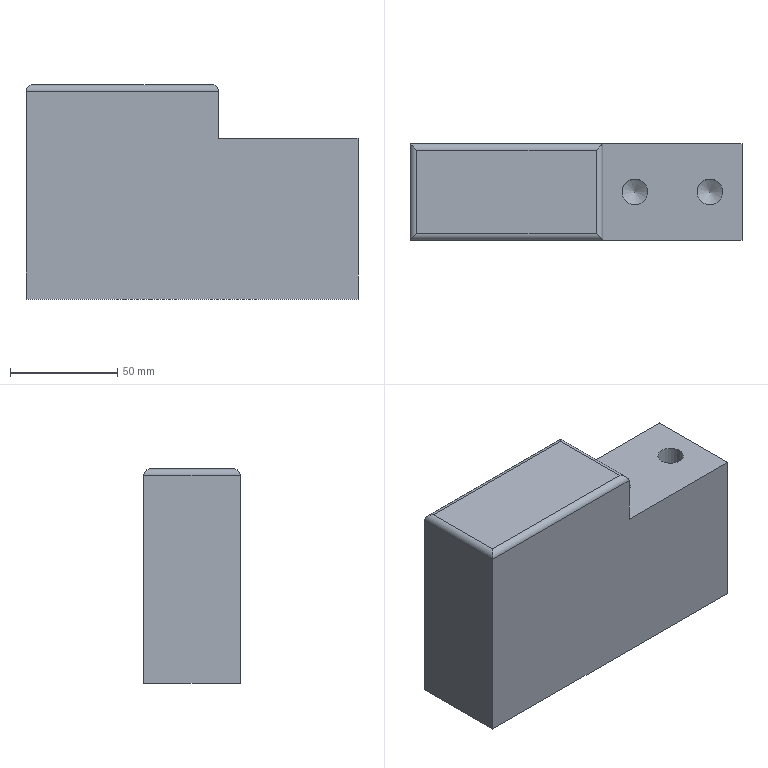Part | NX | features solid 2 | 1 solid | 16 faces | box 155 x 45 x 100 mm | volume 615675 mm3 | plane 8 | cylinder 6 | cone 2 | commonest cylinder face diameters 6 x4 12 x2
STEP:
#1=CARTESIAN_POINT('',(-440.,328.5,305.));
#2=VERTEX_POINT('',#1);
#3=CARTESIAN_POINT('',(-595.,328.5,305.));
#4=VERTEX_POINT('',#3);
#5=CARTESIAN_POINT('',(-440.,328.5,305.));
#6=DIRECTION('',(-1.,0.,0.));
#7=VECTOR('',#6,1000.);
#8=LINE('',#5,#7);
#9=EDGE_CURVE('',#2,#4,#8,.T.);
#10=ORIENTED_EDGE('',*,*,#9,.F.);
#11=CARTESIAN_POINT('',(-440.,283.5,305.));
#12=VERTEX_POINT('',#11);
#13=CARTESIAN_POINT('',(-440.,263.5,305.));
#14=DIRECTION('',(0.,1.,0.));
#15=VECTOR('',#14,1000.);
#16=LINE('',#13,#15);
#17=EDGE_CURVE('',#12,#2,#16,.T.);
#18=ORIENTED_EDGE('',*,*,#17,.F.);
#19=CARTESIAN_POINT('',(-595.,283.5,305.));
#20=VERTEX_POINT('',#19);
#21=CARTESIAN_POINT('',(-605.,283.5,305.));
#22=DIRECTION('',(1.,0.,0.));
#23=VECTOR('',#22,1000.);
#24=LINE('',#21,#23);
#25=EDGE_CURVE('',#20,#12,#24,.T.);
#26=ORIENTED_EDGE('',*,*,#25,.F.);
#27=CARTESIAN_POINT('',(-595.,328.5,305.));
#28=DIRECTION('',(0.,-1.,0.));
#29=VECTOR('',#28,1000.);
#30=LINE('',#27,#29);
#31=EDGE_CURVE('',#4,#20,#30,.T.);
#32=ORIENTED_EDGE('',*,*,#31,.F.);
#33=EDGE_LOOP('',(#10,#18,#26,#32));
#34=FACE_BOUND('',#33,.T.);
#35=CARTESIAN_POINT('',(-440.,98.5,305.));
#36=DIRECTION('',(0.,0.,-1.));
#37=DIRECTION('',(-1.,0.,0.));
#38=AXIS2_PLACEMENT_3D('',#35,#36,#37);
#39=PLANE('',#38);
#40=ADVANCED_FACE('',(#34),#39,.T.);
#41=CARTESIAN_POINT('',(-592.,325.5,405.));
#42=VERTEX_POINT('',#41);
#43=CARTESIAN_POINT('',(-508.,325.5,405.));
#44=VERTEX_POINT('',#43);
#45=CARTESIAN_POINT('',(-440.,325.5,405.));
#46=DIRECTION('',(-1.,0.,0.));
#47=VECTOR('',#46,1000.);
#48=LINE('',#45,#47);
#49=EDGE_CURVE('',#42,#44,#48,.F.);
#50=ORIENTED_EDGE('',*,*,#49,.F.);
#51=CARTESIAN_POINT('',(-592.,286.5,405.));
#52=VERTEX_POINT('',#51);
#53=CARTESIAN_POINT('',(-592.,98.5,405.));
#54=DIRECTION('',(0.,-1.,0.));
#55=VECTOR('',#54,1000.);
#56=LINE('',#53,#55);
#57=EDGE_CURVE('',#52,#42,#56,.F.);
#58=ORIENTED_EDGE('',*,*,#57,.F.);
#59=CARTESIAN_POINT('',(-508.,286.5,405.));
#60=VERTEX_POINT('',#59);
#61=CARTESIAN_POINT('',(-440.,286.5,405.));
#62=DIRECTION('',(1.,0.,0.));
#63=VECTOR('',#62,1000.);
#64=LINE('',#61,#63);
#65=EDGE_CURVE('',#60,#52,#64,.F.);
#66=ORIENTED_EDGE('',*,*,#65,.F.);
#67=CARTESIAN_POINT('',(-508.,98.5,405.));
#68=DIRECTION('',(0.,1.,0.));
#69=VECTOR('',#68,1000.);
#70=LINE('',#67,#69);
#71=EDGE_CURVE('',#44,#60,#70,.F.);
#72=ORIENTED_EDGE('',*,*,#71,.F.);
#73=EDGE_LOOP('',(#50,#58,#66,#72));
#74=FACE_BOUND('',#73,.T.);
#75=CARTESIAN_POINT('',(-440.,98.5,405.));
#76=DIRECTION('',(0.,0.,-1.));
#77=DIRECTION('',(-1.,0.,0.));
#78=AXIS2_PLACEMENT_3D('',#75,#76,#77);
#79=PLANE('',#78);
#80=ADVANCED_FACE('',(#74),#79,.F.);
#81=CARTESIAN_POINT('',(-505.,328.5,380.));
#82=VERTEX_POINT('',#81);
#83=CARTESIAN_POINT('',(-505.,328.5,402.));
#84=VERTEX_POINT('',#83);
#85=CARTESIAN_POINT('',(-505.,328.5,380.));
#86=DIRECTION('',(0.,0.,1.));
#87=VECTOR('',#86,1000.);
#88=LINE('',#85,#87);
#89=EDGE_CURVE('',#82,#84,#88,.T.);
#90=ORIENTED_EDGE('',*,*,#89,.F.);
#91=CARTESIAN_POINT('',(-440.,328.5,380.));
#92=VERTEX_POINT('',#91);
#93=CARTESIAN_POINT('',(-440.,328.5,380.));
#94=DIRECTION('',(-1.,0.,0.));
#95=VECTOR('',#94,1000.);
#96=LINE('',#93,#95);
#97=EDGE_CURVE('',#92,#82,#96,.T.);
#98=ORIENTED_EDGE('',*,*,#97,.F.);
#99=CARTESIAN_POINT('',(-440.,328.5,320.));
#100=DIRECTION('',(0.,0.,1.));
#101=VECTOR('',#100,1000.);
#102=LINE('',#99,#101);
#103=EDGE_CURVE('',#2,#92,#102,.T.);
#104=ORIENTED_EDGE('',*,*,#103,.F.);
#105=ORIENTED_EDGE('',*,*,#9,.T.);
#106=CARTESIAN_POINT('',(-595.,328.5,402.));
#107=VERTEX_POINT('',#106);
#108=CARTESIAN_POINT('',(-595.,328.5,320.));
#109=DIRECTION('',(0.,0.,1.));
#110=VECTOR('',#109,1000.);
#111=LINE('',#108,#110);
#112=EDGE_CURVE('',#4,#107,#111,.T.);
#113=ORIENTED_EDGE('',*,*,#112,.T.);
#114=CARTESIAN_POINT('',(-440.,328.5,402.));
#115=DIRECTION('',(-1.,0.,0.));
#116=VECTOR('',#115,1000.);
#117=LINE('',#114,#116);
#118=EDGE_CURVE('',#84,#107,#117,.T.);
#119=ORIENTED_EDGE('',*,*,#118,.F.);
#120=EDGE_LOOP('',(#90,#98,#104,#105,#113,#119));
#121=FACE_BOUND('',#120,.T.);
#122=CARTESIAN_POINT('',(-440.,328.5,320.));
#123=DIRECTION('',(0.,-1.,0.));
#124=DIRECTION('',(0.,0.,1.));
#125=AXIS2_PLACEMENT_3D('',#122,#123,#124);
#126=PLANE('',#125);
#127=ADVANCED_FACE('',(#121),#126,.F.);
#128=CARTESIAN_POINT('',(-595.,283.5,402.));
#129=VERTEX_POINT('',#128);
#130=CARTESIAN_POINT('',(-595.,283.5,320.));
#131=DIRECTION('',(0.,0.,-1.));
#132=VECTOR('',#131,1000.);
#133=LINE('',#130,#132);
#134=EDGE_CURVE('',#129,#20,#133,.T.);
#135=ORIENTED_EDGE('',*,*,#134,.T.);
#136=ORIENTED_EDGE('',*,*,#25,.T.);
#137=CARTESIAN_POINT('',(-440.,283.5,380.));
#138=VERTEX_POINT('',#137);
#139=CARTESIAN_POINT('',(-440.,283.5,320.));
#140=DIRECTION('',(0.,0.,1.));
#141=VECTOR('',#140,1000.);
#142=LINE('',#139,#141);
#143=EDGE_CURVE('',#12,#138,#142,.T.);
#144=ORIENTED_EDGE('',*,*,#143,.T.);
#145=CARTESIAN_POINT('',(-505.,283.5,380.));
#146=VERTEX_POINT('',#145);
#147=CARTESIAN_POINT('',(-440.,283.5,380.));
#148=DIRECTION('',(-1.,0.,0.));
#149=VECTOR('',#148,1000.);
#150=LINE('',#147,#149);
#151=EDGE_CURVE('',#138,#146,#150,.T.);
#152=ORIENTED_EDGE('',*,*,#151,.T.);
#153=CARTESIAN_POINT('',(-505.,283.5,402.));
#154=VERTEX_POINT('',#153);
#155=CARTESIAN_POINT('',(-505.,283.5,380.));
#156=DIRECTION('',(0.,0.,1.));
#157=VECTOR('',#156,1000.);
#158=LINE('',#155,#157);
#159=EDGE_CURVE('',#146,#154,#158,.T.);
#160=ORIENTED_EDGE('',*,*,#159,.T.);
#161=CARTESIAN_POINT('',(-605.,283.5,402.));
#162=DIRECTION('',(1.,0.,0.));
#163=VECTOR('',#162,1000.);
#164=LINE('',#161,#163);
#165=EDGE_CURVE('',#129,#154,#164,.T.);
#166=ORIENTED_EDGE('',*,*,#165,.F.);
#167=EDGE_LOOP('',(#135,#136,#144,#152,#160,#166));
#168=FACE_BOUND('',#167,.T.);
#169=CARTESIAN_POINT('',(-605.,283.5,320.));
#170=DIRECTION('',(0.,1.,0.));
#171=DIRECTION('',(0.,0.,-1.));
#172=AXIS2_PLACEMENT_3D('',#169,#170,#171);
#173=PLANE('',#172);
#174=ADVANCED_FACE('',(#168),#173,.F.);
#175=ORIENTED_EDGE('',*,*,#159,.F.);
#176=CARTESIAN_POINT('',(-505.,263.5,380.));
#177=DIRECTION('',(0.,-1.,0.));
#178=VECTOR('',#177,1000.);
#179=LINE('',#176,#178);
#180=EDGE_CURVE('',#146,#82,#179,.F.);
#181=ORIENTED_EDGE('',*,*,#180,.T.);
#182=ORIENTED_EDGE('',*,*,#89,.T.);
#183=CARTESIAN_POINT('',(-505.,263.5,402.));
#184=DIRECTION('',(0.,1.,0.));
#185=VECTOR('',#184,1000.);
#186=LINE('',#183,#185);
#187=EDGE_CURVE('',#154,#84,#186,.T.);
#188=ORIENTED_EDGE('',*,*,#187,.F.);
#189=EDGE_LOOP('',(#175,#181,#182,#188));
#190=FACE_BOUND('',#189,.T.);
#191=CARTESIAN_POINT('',(-505.,263.5,380.));
#192=DIRECTION('',(-1.,0.,0.));
#193=DIRECTION('',(0.,0.,1.));
#194=AXIS2_PLACEMENT_3D('',#191,#192,#193);
#195=PLANE('',#194);
#196=ADVANCED_FACE('',(#190),#195,.F.);
#197=ORIENTED_EDGE('',*,*,#143,.F.);
#198=ORIENTED_EDGE('',*,*,#17,.T.);
#199=ORIENTED_EDGE('',*,*,#103,.T.);
#200=CARTESIAN_POINT('',(-440.,263.5,380.));
#201=DIRECTION('',(0.,1.,0.));
#202=VECTOR('',#201,1000.);
#203=LINE('',#200,#202);
#204=EDGE_CURVE('',#138,#92,#203,.T.);
#205=ORIENTED_EDGE('',*,*,#204,.F.);
#206=EDGE_LOOP('',(#197,#198,#199,#205));
#207=FACE_BOUND('',#206,.T.);
#208=CARTESIAN_POINT('',(-440.,263.5,320.));
#209=DIRECTION('',(-1.,0.,0.));
#210=DIRECTION('',(0.,0.,1.));
#211=AXIS2_PLACEMENT_3D('',#208,#209,#210);
#212=PLANE('',#211);
#213=ADVANCED_FACE('',(#207),#212,.F.);
#214=CARTESIAN_POINT('',(-496.,306.,345.));
#215=VERTEX_POINT('',#214);
#216=CARTESIAN_POINT('',(-490.,306.,345.));
#217=DIRECTION('',(0.,0.,-1.));
#218=DIRECTION('',(-1.,0.,0.));
#219=AXIS2_PLACEMENT_3D('',#216,#217,#218);
#220=CIRCLE('',#219,6.);
#221=EDGE_CURVE('',#215,#215,#220,.T.);
#222=ORIENTED_EDGE('',*,*,#221,.T.);
#223=EDGE_LOOP('',(#222));
#224=FACE_BOUND('',#223,.T.);
#225=CARTESIAN_POINT('',(-484.,306.,380.));
#226=VERTEX_POINT('',#225);
#227=CARTESIAN_POINT('',(-490.,306.,380.));
#228=DIRECTION('',(0.,0.,1.));
#229=DIRECTION('',(1.,0.,0.));
#230=AXIS2_PLACEMENT_3D('',#227,#228,#229);
#231=CIRCLE('',#230,6.);
#232=EDGE_CURVE('',#226,#226,#231,.T.);
#233=ORIENTED_EDGE('',*,*,#232,.T.);
#234=EDGE_LOOP('',(#233));
#235=FACE_BOUND('',#234,.T.);
#236=CARTESIAN_POINT('',(-490.,306.,395.));
#237=DIRECTION('',(0.,0.,-1.));
#238=DIRECTION('',(-1.,0.,0.));
#239=AXIS2_PLACEMENT_3D('',#236,#237,#238);
#240=CYLINDRICAL_SURFACE('',#239,6.);
#241=ADVANCED_FACE('',(#224,#235),#240,.F.);
#242=CARTESIAN_POINT('',(-461.,306.,380.));
#243=VERTEX_POINT('',#242);
#244=CARTESIAN_POINT('',(-455.,306.,380.));
#245=DIRECTION('',(0.,0.,1.));
#246=DIRECTION('',(-1.,0.,0.));
#247=AXIS2_PLACEMENT_3D('',#244,#245,#246);
#248=CIRCLE('',#247,6.);
#249=EDGE_CURVE('',#243,#243,#248,.T.);
#250=ORIENTED_EDGE('',*,*,#249,.F.);
#251=EDGE_LOOP('',(#250));
#252=FACE_BOUND('',#251,.T.);
#253=ORIENTED_EDGE('',*,*,#232,.F.);
#254=EDGE_LOOP('',(#253));
#255=FACE_BOUND('',#254,.T.);
#256=ORIENTED_EDGE('',*,*,#151,.F.);
#257=ORIENTED_EDGE('',*,*,#204,.T.);
#258=ORIENTED_EDGE('',*,*,#97,.T.);
#259=ORIENTED_EDGE('',*,*,#180,.F.);
#260=EDGE_LOOP('',(#256,#257,#258,#259));
#261=FACE_BOUND('',#260,.T.);
#262=CARTESIAN_POINT('',(-440.,263.5,380.));
#263=DIRECTION('',(0.,0.,-1.));
#264=DIRECTION('',(0.,1.,0.));
#265=AXIS2_PLACEMENT_3D('',#262,#263,#264);
#266=PLANE('',#265);
#267=ADVANCED_FACE('',(#252,#255,#261),#266,.F.);
#268=CARTESIAN_POINT('',(-461.,306.,345.));
#269=VERTEX_POINT('',#268);
#270=CARTESIAN_POINT('',(-455.,306.,345.));
#271=DIRECTION('',(0.,0.,-1.));
#272=DIRECTION('',(-1.,0.,0.));
#273=AXIS2_PLACEMENT_3D('',#270,#271,#272);
#274=CIRCLE('',#273,6.);
#275=EDGE_CURVE('',#269,#269,#274,.T.);
#276=ORIENTED_EDGE('',*,*,#275,.T.);
#277=EDGE_LOOP('',(#276));
#278=FACE_BOUND('',#277,.T.);
#279=ORIENTED_EDGE('',*,*,#249,.T.);
#280=EDGE_LOOP('',(#279));
#281=FACE_BOUND('',#280,.T.);
#282=CARTESIAN_POINT('',(-455.,306.,380.));
#283=DIRECTION('',(0.,0.,-1.));
#284=DIRECTION('',(-1.,0.,0.));
#285=AXIS2_PLACEMENT_3D('',#282,#283,#284);
#286=CYLINDRICAL_SURFACE('',#285,6.);
#287=ADVANCED_FACE('',(#278,#281),#286,.F.);
#288=ORIENTED_EDGE('',*,*,#221,.F.);
#289=EDGE_LOOP('',(#288));
#290=FACE_BOUND('',#289,.T.);
#291=CARTESIAN_POINT('',(-490.,306.,341.395));
#292=VERTEX_POINT('',#291);
#293=VERTEX_LOOP('',#292);
#294=FACE_BOUND('',#293,.T.);
#295=CARTESIAN_POINT('',(-490.,306.,345.));
#296=DIRECTION('',(0.,0.,1.));
#297=DIRECTION('',(1.,0.,0.));
#298=AXIS2_PLACEMENT_3D('',#295,#296,#297);
#299=CONICAL_SURFACE('',#298,6.,1.03);
#300=ADVANCED_FACE('',(#290,#294),#299,.F.);
#301=ORIENTED_EDGE('',*,*,#275,.F.);
#302=EDGE_LOOP('',(#301));
#303=FACE_BOUND('',#302,.T.);
#304=CARTESIAN_POINT('',(-455.,306.,341.395));
#305=VERTEX_POINT('',#304);
#306=VERTEX_LOOP('',#305);
#307=FACE_BOUND('',#306,.T.);
#308=CARTESIAN_POINT('',(-455.,306.,345.));
#309=DIRECTION('',(0.,0.,1.));
#310=DIRECTION('',(1.,0.,0.));
#311=AXIS2_PLACEMENT_3D('',#308,#309,#310);
#312=CONICAL_SURFACE('',#311,6.,1.03);
#313=ADVANCED_FACE('',(#303,#307),#312,.F.);
#314=ORIENTED_EDGE('',*,*,#112,.F.);
#315=ORIENTED_EDGE('',*,*,#31,.T.);
#316=ORIENTED_EDGE('',*,*,#134,.F.);
#317=CARTESIAN_POINT('',(-595.,328.5,402.));
#318=DIRECTION('',(0.,-1.,0.));
#319=VECTOR('',#318,1000.);
#320=LINE('',#317,#319);
#321=EDGE_CURVE('',#107,#129,#320,.T.);
#322=ORIENTED_EDGE('',*,*,#321,.F.);
#323=EDGE_LOOP('',(#314,#315,#316,#322));
#324=FACE_BOUND('',#323,.T.);
#325=CARTESIAN_POINT('',(-595.,328.5,320.));
#326=DIRECTION('',(1.,0.,0.));
#327=DIRECTION('',(0.,0.,-1.));
#328=AXIS2_PLACEMENT_3D('',#325,#326,#327);
#329=PLANE('',#328);
#330=ADVANCED_FACE('',(#324),#329,.F.);
#331=CARTESIAN_POINT('',(-592.,325.5,402.));
#332=DIRECTION('',(0.7071,0.7071,0.));
#333=DIRECTION('',(-0.7071,0.7071,0.));
#334=AXIS2_PLACEMENT_3D('',#331,#332,#333);
#335=ELLIPSE('',#334,4.243,3.);
#336=EDGE_CURVE('',#42,#107,#335,.F.);
#337=ORIENTED_EDGE('',*,*,#336,.T.);
#338=ORIENTED_EDGE('',*,*,#321,.T.);
#339=CARTESIAN_POINT('',(-592.,286.5,402.));
#340=DIRECTION('',(-0.7071,0.7071,0.));
#341=DIRECTION('',(-0.7071,-0.7071,0.));
#342=AXIS2_PLACEMENT_3D('',#339,#340,#341);
#343=ELLIPSE('',#342,4.243,3.);
#344=EDGE_CURVE('',#129,#52,#343,.T.);
#345=ORIENTED_EDGE('',*,*,#344,.T.);
#346=ORIENTED_EDGE('',*,*,#57,.T.);
#347=EDGE_LOOP('',(#337,#338,#345,#346));
#348=FACE_BOUND('',#347,.T.);
#349=CARTESIAN_POINT('',(-592.,328.5,402.));
#350=DIRECTION('',(0.,-1.,0.));
#351=DIRECTION('',(0.,0.,-1.));
#352=AXIS2_PLACEMENT_3D('',#349,#350,#351);
#353=CYLINDRICAL_SURFACE('',#352,3.);
#354=ADVANCED_FACE('',(#348),#353,.T.);
#355=ORIENTED_EDGE('',*,*,#344,.F.);
#356=ORIENTED_EDGE('',*,*,#165,.T.);
#357=CARTESIAN_POINT('',(-508.,286.5,402.));
#358=DIRECTION('',(-0.7071,-0.7071,0.));
#359=DIRECTION('',(0.7071,-0.7071,0.));
#360=AXIS2_PLACEMENT_3D('',#357,#358,#359);
#361=ELLIPSE('',#360,4.243,3.);
#362=EDGE_CURVE('',#154,#60,#361,.T.);
#363=ORIENTED_EDGE('',*,*,#362,.T.);
#364=ORIENTED_EDGE('',*,*,#65,.T.);
#365=EDGE_LOOP('',(#355,#356,#363,#364));
#366=FACE_BOUND('',#365,.T.);
#367=CARTESIAN_POINT('',(-605.,286.5,402.));
#368=DIRECTION('',(1.,0.,0.));
#369=DIRECTION('',(0.,0.,1.));
#370=AXIS2_PLACEMENT_3D('',#367,#368,#369);
#371=CYLINDRICAL_SURFACE('',#370,3.);
#372=ADVANCED_FACE('',(#366),#371,.T.);
#373=ORIENTED_EDGE('',*,*,#336,.F.);
#374=ORIENTED_EDGE('',*,*,#49,.T.);
#375=CARTESIAN_POINT('',(-508.,325.5,402.));
#376=DIRECTION('',(0.7071,-0.7071,0.));
#377=DIRECTION('',(-0.7071,-0.7071,0.));
#378=AXIS2_PLACEMENT_3D('',#375,#376,#377);
#379=ELLIPSE('',#378,4.243,3.);
#380=EDGE_CURVE('',#44,#84,#379,.F.);
#381=ORIENTED_EDGE('',*,*,#380,.T.);
#382=ORIENTED_EDGE('',*,*,#118,.T.);
#383=EDGE_LOOP('',(#373,#374,#381,#382));
#384=FACE_BOUND('',#383,.T.);
#385=CARTESIAN_POINT('',(-440.,325.5,402.));
#386=DIRECTION('',(-1.,0.,0.));
#387=DIRECTION('',(0.,0.,-1.));
#388=AXIS2_PLACEMENT_3D('',#385,#386,#387);
#389=CYLINDRICAL_SURFACE('',#388,3.);
#390=ADVANCED_FACE('',(#384),#389,.T.);
#391=ORIENTED_EDGE('',*,*,#362,.F.);
#392=ORIENTED_EDGE('',*,*,#187,.T.);
#393=ORIENTED_EDGE('',*,*,#380,.F.);
#394=ORIENTED_EDGE('',*,*,#71,.T.);
#395=EDGE_LOOP('',(#391,#392,#393,#394));
#396=FACE_BOUND('',#395,.T.);
#397=CARTESIAN_POINT('',(-508.,263.5,402.));
#398=DIRECTION('',(0.,1.,0.));
#399=DIRECTION('',(0.,0.,1.));
#400=AXIS2_PLACEMENT_3D('',#397,#398,#399);
#401=CYLINDRICAL_SURFACE('',#400,3.);
#402=ADVANCED_FACE('',(#396),#401,.T.);
#403=CLOSED_SHELL('',(#40,#80,#127,#174,#196,#213,#241,#267,#287,#300,#313,#330,#354,#372,#390,#402));
#404=MANIFOLD_SOLID_BREP('',#403);
#405=(LENGTH_UNIT()NAMED_UNIT(*)SI_UNIT(.MILLI.,.METRE.));
#406=UNCERTAINTY_MEASURE_WITH_UNIT(LENGTH_MEASURE(0.00001),#405,'','');
#407=(NAMED_UNIT(*)PLANE_ANGLE_UNIT()SI_UNIT($,.RADIAN.));
#408=(NAMED_UNIT(*)SI_UNIT($,.STERADIAN.)SOLID_ANGLE_UNIT());
#409=(GEOMETRIC_REPRESENTATION_CONTEXT(3)GLOBAL_UNCERTAINTY_ASSIGNED_CONTEXT((#406))GLOBAL_UNIT_ASSIGNED_CONTEXT((#405,#407,#408))REPRESENTATION_CONTEXT('',''));
#410=ADVANCED_BREP_SHAPE_REPRESENTATION('',(#404),#409);